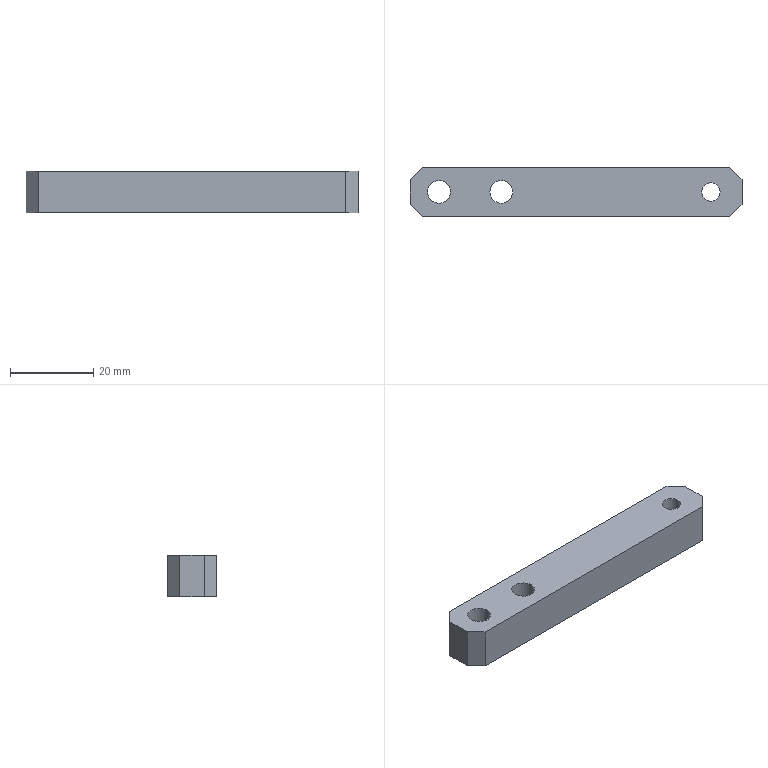Part | STEP file | 11-FG-B06711 | 1 solid | 27 faces | box 80 x 12 x 10 mm | volume 7960 mm3 | cylinder 14 | plane 13 | commonest cylinder face diameters 5.5 x4 10 x4 3.3 x2 4.4 x2 8 x2
STEP:
#1=CARTESIAN_POINT('',(12.,6.,5.4));
#2=VERTEX_POINT('',#1);
#3=CARTESIAN_POINT('',(2.,6.,5.4));
#4=VERTEX_POINT('',#3);
#5=CARTESIAN_POINT('',(7.,6.,5.4));
#6=DIRECTION('',(0.,0.,-1.));
#7=DIRECTION('',(-1.,0.,0.));
#8=AXIS2_PLACEMENT_3D('',#5,#6,#7);
#9=CIRCLE('',#8,5.);
#10=EDGE_CURVE('',#2,#4,#9,.T.);
#11=ORIENTED_EDGE('',*,*,#10,.F.);
#12=CARTESIAN_POINT('',(12.,6.,0.));
#13=VERTEX_POINT('',#12);
#14=CARTESIAN_POINT('',(12.,6.,0.));
#15=DIRECTION('',(0.,0.,-1.));
#16=VECTOR('',#15,1000.);
#17=LINE('',#14,#16);
#18=EDGE_CURVE('',#2,#13,#17,.T.);
#19=ORIENTED_EDGE('',*,*,#18,.T.);
#20=CARTESIAN_POINT('',(2.,6.,0.));
#21=VERTEX_POINT('',#20);
#22=CARTESIAN_POINT('',(7.,6.,0.));
#23=DIRECTION('',(0.,0.,-1.));
#24=DIRECTION('',(-1.,0.,0.));
#25=AXIS2_PLACEMENT_3D('',#22,#23,#24);
#26=CIRCLE('',#25,5.);
#27=EDGE_CURVE('',#13,#21,#26,.T.);
#28=ORIENTED_EDGE('',*,*,#27,.T.);
#29=CARTESIAN_POINT('',(2.,6.,0.));
#30=DIRECTION('',(0.,0.,-1.));
#31=VECTOR('',#30,1000.);
#32=LINE('',#29,#31);
#33=EDGE_CURVE('',#4,#21,#32,.T.);
#34=ORIENTED_EDGE('',*,*,#33,.F.);
#35=EDGE_LOOP('',(#11,#19,#28,#34));
#36=FACE_OUTER_BOUND('',#35,.T.);
#37=CARTESIAN_POINT('',(7.,6.,0.));
#38=DIRECTION('',(0.,0.,-1.));
#39=DIRECTION('',(-1.,0.,0.));
#40=AXIS2_PLACEMENT_3D('',#37,#38,#39);
#41=CYLINDRICAL_SURFACE('',#40,5.);
#42=ADVANCED_FACE('',(#36),#41,.F.);
#43=CARTESIAN_POINT('',(9.75,6.,10.));
#44=VERTEX_POINT('',#43);
#45=CARTESIAN_POINT('',(4.25,6.,10.));
#46=VERTEX_POINT('',#45);
#47=CARTESIAN_POINT('',(7.,6.,10.));
#48=DIRECTION('',(0.,0.,-1.));
#49=DIRECTION('',(-1.,0.,0.));
#50=AXIS2_PLACEMENT_3D('',#47,#48,#49);
#51=CIRCLE('',#50,2.75);
#52=EDGE_CURVE('',#44,#46,#51,.T.);
#53=ORIENTED_EDGE('',*,*,#52,.F.);
#54=CARTESIAN_POINT('',(9.75,6.,5.4));
#55=VERTEX_POINT('',#54);
#56=CARTESIAN_POINT('',(9.75,6.,0.));
#57=DIRECTION('',(0.,0.,-1.));
#58=VECTOR('',#57,1000.);
#59=LINE('',#56,#58);
#60=EDGE_CURVE('',#44,#55,#59,.T.);
#61=ORIENTED_EDGE('',*,*,#60,.T.);
#62=CARTESIAN_POINT('',(4.25,6.,5.4));
#63=VERTEX_POINT('',#62);
#64=CARTESIAN_POINT('',(7.,6.,5.4));
#65=DIRECTION('',(0.,0.,-1.));
#66=DIRECTION('',(-1.,0.,0.));
#67=AXIS2_PLACEMENT_3D('',#64,#65,#66);
#68=CIRCLE('',#67,2.75);
#69=EDGE_CURVE('',#55,#63,#68,.T.);
#70=ORIENTED_EDGE('',*,*,#69,.T.);
#71=CARTESIAN_POINT('',(4.25,6.,0.));
#72=DIRECTION('',(0.,0.,-1.));
#73=VECTOR('',#72,1000.);
#74=LINE('',#71,#73);
#75=EDGE_CURVE('',#46,#63,#74,.T.);
#76=ORIENTED_EDGE('',*,*,#75,.F.);
#77=EDGE_LOOP('',(#53,#61,#70,#76));
#78=FACE_OUTER_BOUND('',#77,.T.);
#79=CARTESIAN_POINT('',(7.,6.,0.));
#80=DIRECTION('',(0.,0.,-1.));
#81=DIRECTION('',(-1.,0.,0.));
#82=AXIS2_PLACEMENT_3D('',#79,#80,#81);
#83=CYLINDRICAL_SURFACE('',#82,2.75);
#84=ADVANCED_FACE('',(#78),#83,.F.);
#85=CARTESIAN_POINT('',(27.,6.,5.4));
#86=VERTEX_POINT('',#85);
#87=CARTESIAN_POINT('',(17.,6.,5.4));
#88=VERTEX_POINT('',#87);
#89=CARTESIAN_POINT('',(22.,6.,5.4));
#90=DIRECTION('',(0.,0.,-1.));
#91=DIRECTION('',(-1.,0.,0.));
#92=AXIS2_PLACEMENT_3D('',#89,#90,#91);
#93=CIRCLE('',#92,5.);
#94=EDGE_CURVE('',#86,#88,#93,.T.);
#95=ORIENTED_EDGE('',*,*,#94,.F.);
#96=CARTESIAN_POINT('',(27.,6.,0.));
#97=VERTEX_POINT('',#96);
#98=CARTESIAN_POINT('',(27.,6.,0.));
#99=DIRECTION('',(0.,0.,-1.));
#100=VECTOR('',#99,1000.);
#101=LINE('',#98,#100);
#102=EDGE_CURVE('',#86,#97,#101,.T.);
#103=ORIENTED_EDGE('',*,*,#102,.T.);
#104=CARTESIAN_POINT('',(17.,6.,0.));
#105=VERTEX_POINT('',#104);
#106=CARTESIAN_POINT('',(22.,6.,0.));
#107=DIRECTION('',(0.,0.,-1.));
#108=DIRECTION('',(-1.,0.,0.));
#109=AXIS2_PLACEMENT_3D('',#106,#107,#108);
#110=CIRCLE('',#109,5.);
#111=EDGE_CURVE('',#97,#105,#110,.T.);
#112=ORIENTED_EDGE('',*,*,#111,.T.);
#113=CARTESIAN_POINT('',(17.,6.,0.));
#114=DIRECTION('',(0.,0.,-1.));
#115=VECTOR('',#114,1000.);
#116=LINE('',#113,#115);
#117=EDGE_CURVE('',#88,#105,#116,.T.);
#118=ORIENTED_EDGE('',*,*,#117,.F.);
#119=EDGE_LOOP('',(#95,#103,#112,#118));
#120=FACE_OUTER_BOUND('',#119,.T.);
#121=CARTESIAN_POINT('',(22.,6.,0.));
#122=DIRECTION('',(0.,0.,-1.));
#123=DIRECTION('',(-1.,0.,0.));
#124=AXIS2_PLACEMENT_3D('',#121,#122,#123);
#125=CYLINDRICAL_SURFACE('',#124,5.);
#126=ADVANCED_FACE('',(#120),#125,.F.);
#127=CARTESIAN_POINT('',(24.75,6.,10.));
#128=VERTEX_POINT('',#127);
#129=CARTESIAN_POINT('',(19.25,6.,10.));
#130=VERTEX_POINT('',#129);
#131=CARTESIAN_POINT('',(22.,6.,10.));
#132=DIRECTION('',(0.,0.,-1.));
#133=DIRECTION('',(-1.,0.,0.));
#134=AXIS2_PLACEMENT_3D('',#131,#132,#133);
#135=CIRCLE('',#134,2.75);
#136=EDGE_CURVE('',#128,#130,#135,.T.);
#137=ORIENTED_EDGE('',*,*,#136,.F.);
#138=CARTESIAN_POINT('',(24.75,6.,5.4));
#139=VERTEX_POINT('',#138);
#140=CARTESIAN_POINT('',(24.75,6.,0.));
#141=DIRECTION('',(0.,0.,-1.));
#142=VECTOR('',#141,1000.);
#143=LINE('',#140,#142);
#144=EDGE_CURVE('',#128,#139,#143,.T.);
#145=ORIENTED_EDGE('',*,*,#144,.T.);
#146=CARTESIAN_POINT('',(19.25,6.,5.4));
#147=VERTEX_POINT('',#146);
#148=CARTESIAN_POINT('',(22.,6.,5.4));
#149=DIRECTION('',(0.,0.,-1.));
#150=DIRECTION('',(-1.,0.,0.));
#151=AXIS2_PLACEMENT_3D('',#148,#149,#150);
#152=CIRCLE('',#151,2.75);
#153=EDGE_CURVE('',#139,#147,#152,.T.);
#154=ORIENTED_EDGE('',*,*,#153,.T.);
#155=CARTESIAN_POINT('',(19.25,6.,0.));
#156=DIRECTION('',(0.,0.,-1.));
#157=VECTOR('',#156,1000.);
#158=LINE('',#155,#157);
#159=EDGE_CURVE('',#130,#147,#158,.T.);
#160=ORIENTED_EDGE('',*,*,#159,.F.);
#161=EDGE_LOOP('',(#137,#145,#154,#160));
#162=FACE_OUTER_BOUND('',#161,.T.);
#163=CARTESIAN_POINT('',(22.,6.,0.));
#164=DIRECTION('',(0.,0.,-1.));
#165=DIRECTION('',(-1.,0.,0.));
#166=AXIS2_PLACEMENT_3D('',#163,#164,#165);
#167=CYLINDRICAL_SURFACE('',#166,2.75);
#168=ADVANCED_FACE('',(#162),#167,.F.);
#169=CARTESIAN_POINT('',(76.5,6.,5.15));
#170=VERTEX_POINT('',#169);
#171=CARTESIAN_POINT('',(76.5,6.,1.85));
#172=VERTEX_POINT('',#171);
#173=CARTESIAN_POINT('',(76.5,6.,5.15));
#174=CARTESIAN_POINT('',(76.5,5.891,5.15));
#175=CARTESIAN_POINT('',(76.495,5.781,5.139));
#176=CARTESIAN_POINT('',(76.478,5.567,5.096));
#177=CARTESIAN_POINT('',(76.465,5.464,5.064));
#178=CARTESIAN_POINT('',(76.417,5.165,4.939));
#179=CARTESIAN_POINT('',(76.372,4.984,4.818));
#180=CARTESIAN_POINT('',(76.303,4.756,4.59));
#181=CARTESIAN_POINT('',(76.28,4.689,4.508));
#182=CARTESIAN_POINT('',(76.236,4.57,4.33));
#183=CARTESIAN_POINT('',(76.216,4.519,4.234));
#184=CARTESIAN_POINT('',(76.182,4.436,4.035));
#185=CARTESIAN_POINT('',(76.168,4.404,3.933));
#186=CARTESIAN_POINT('',(76.149,4.361,3.72));
#187=CARTESIAN_POINT('',(76.144,4.35,3.609));
#188=CARTESIAN_POINT('',(76.144,4.35,3.283));
#189=CARTESIAN_POINT('',(76.165,4.394,3.064));
#190=CARTESIAN_POINT('',(76.216,4.518,2.766));
#191=CARTESIAN_POINT('',(76.236,4.57,2.67));
#192=CARTESIAN_POINT('',(76.28,4.689,2.492));
#193=CARTESIAN_POINT('',(76.303,4.757,2.41));
#194=CARTESIAN_POINT('',(76.349,4.908,2.258));
#195=CARTESIAN_POINT('',(76.372,4.992,2.189));
#196=CARTESIAN_POINT('',(76.414,5.169,2.071));
#197=CARTESIAN_POINT('',(76.433,5.263,2.02));
#198=CARTESIAN_POINT('',(76.482,5.565,1.893));
#199=CARTESIAN_POINT('',(76.5,5.779,1.85));
#200=CARTESIAN_POINT('',(76.5,6.,1.85));
#201=B_SPLINE_CURVE_WITH_KNOTS('',3,(#173,#174,#175,#176,#177,#178,#179,#180,#181,#182,#183,#184,#185,#186,#187,#188,#189,#190,#191,#192,#193,#194,#195,#196,#197,#198,#199,#200),.UNSPECIFIED.,.F.,.F.,(4,2,2,2,2,2,2,2,2,2,2,2,2,4),(0.005218,0.005543,0.005869,0.006521,0.006847,0.007173,0.007499,0.007824,0.008476,0.008802,0.009128,0.009454,0.009779,0.01043),.UNSPECIFIED.);
#202=EDGE_CURVE('',#170,#172,#201,.T.);
#203=ORIENTED_EDGE('',*,*,#202,.F.);
#204=CARTESIAN_POINT('',(80.,6.,5.15));
#205=VERTEX_POINT('',#204);
#206=CARTESIAN_POINT('',(80.,6.,5.15));
#207=DIRECTION('',(1.,0.,0.));
#208=VECTOR('',#207,1000.);
#209=LINE('',#206,#208);
#210=EDGE_CURVE('',#170,#205,#209,.T.);
#211=ORIENTED_EDGE('',*,*,#210,.T.);
#212=CARTESIAN_POINT('',(80.,6.,1.85));
#213=VERTEX_POINT('',#212);
#214=CARTESIAN_POINT('',(80.,6.,3.5));
#215=DIRECTION('',(1.,0.,0.));
#216=DIRECTION('',(0.,0.,-1.));
#217=AXIS2_PLACEMENT_3D('',#214,#215,#216);
#218=CIRCLE('',#217,1.65);
#219=EDGE_CURVE('',#205,#213,#218,.T.);
#220=ORIENTED_EDGE('',*,*,#219,.T.);
#221=CARTESIAN_POINT('',(80.,6.,1.85));
#222=DIRECTION('',(1.,0.,0.));
#223=VECTOR('',#222,1000.);
#224=LINE('',#221,#223);
#225=EDGE_CURVE('',#172,#213,#224,.T.);
#226=ORIENTED_EDGE('',*,*,#225,.F.);
#227=EDGE_LOOP('',(#203,#211,#220,#226));
#228=FACE_OUTER_BOUND('',#227,.T.);
#229=CARTESIAN_POINT('',(80.,6.,3.5));
#230=DIRECTION('',(1.,0.,0.));
#231=DIRECTION('',(0.,0.,-1.));
#232=AXIS2_PLACEMENT_3D('',#229,#230,#231);
#233=CYLINDRICAL_SURFACE('',#232,1.65);
#234=ADVANCED_FACE('',(#228),#233,.F.);
#235=CARTESIAN_POINT('',(74.7,6.,6.));
#236=VERTEX_POINT('',#235);
#237=CARTESIAN_POINT('',(70.3,6.,6.));
#238=VERTEX_POINT('',#237);
#239=CARTESIAN_POINT('',(72.5,6.,6.));
#240=DIRECTION('',(0.,0.,-1.));
#241=DIRECTION('',(-1.,0.,0.));
#242=AXIS2_PLACEMENT_3D('',#239,#240,#241);
#243=CIRCLE('',#242,2.2);
#244=EDGE_CURVE('',#236,#238,#243,.T.);
#245=ORIENTED_EDGE('',*,*,#244,.T.);
#246=CARTESIAN_POINT('',(70.3,6.,10.));
#247=VERTEX_POINT('',#246);
#248=CARTESIAN_POINT('',(70.3,6.,10.));
#249=DIRECTION('',(0.,0.,1.));
#250=VECTOR('',#249,1000.);
#251=LINE('',#248,#250);
#252=EDGE_CURVE('',#238,#247,#251,.T.);
#253=ORIENTED_EDGE('',*,*,#252,.T.);
#254=CARTESIAN_POINT('',(74.7,6.,10.));
#255=VERTEX_POINT('',#254);
#256=CARTESIAN_POINT('',(72.5,6.,10.));
#257=DIRECTION('',(0.,0.,1.));
#258=DIRECTION('',(1.,0.,0.));
#259=AXIS2_PLACEMENT_3D('',#256,#257,#258);
#260=CIRCLE('',#259,2.2);
#261=EDGE_CURVE('',#247,#255,#260,.T.);
#262=ORIENTED_EDGE('',*,*,#261,.T.);
#263=CARTESIAN_POINT('',(74.7,6.,10.));
#264=DIRECTION('',(0.,0.,1.));
#265=VECTOR('',#264,1000.);
#266=LINE('',#263,#265);
#267=EDGE_CURVE('',#236,#255,#266,.T.);
#268=ORIENTED_EDGE('',*,*,#267,.F.);
#269=EDGE_LOOP('',(#245,#253,#262,#268));
#270=FACE_OUTER_BOUND('',#269,.T.);
#271=CARTESIAN_POINT('',(72.5,6.,10.));
#272=DIRECTION('',(0.,0.,1.));
#273=DIRECTION('',(1.,0.,0.));
#274=AXIS2_PLACEMENT_3D('',#271,#272,#273);
#275=CYLINDRICAL_SURFACE('',#274,2.2);
#276=ADVANCED_FACE('',(#270),#275,.F.);
#277=CARTESIAN_POINT('',(76.5,6.,6.));
#278=VERTEX_POINT('',#277);
#279=CARTESIAN_POINT('',(68.5,6.,6.));
#280=VERTEX_POINT('',#279);
#281=CARTESIAN_POINT('',(72.5,6.,6.));
#282=DIRECTION('',(0.,0.,-1.));
#283=DIRECTION('',(-1.,0.,0.));
#284=AXIS2_PLACEMENT_3D('',#281,#282,#283);
#285=CIRCLE('',#284,4.);
#286=EDGE_CURVE('',#278,#280,#285,.T.);
#287=ORIENTED_EDGE('',*,*,#286,.F.);
#288=CARTESIAN_POINT('',(76.5,6.,6.));
#289=DIRECTION('',(0.,0.,-1.));
#290=VECTOR('',#289,1000.);
#291=LINE('',#288,#290);
#292=EDGE_CURVE('',#278,#170,#291,.T.);
#293=ORIENTED_EDGE('',*,*,#292,.T.);
#294=ORIENTED_EDGE('',*,*,#202,.T.);
#295=CARTESIAN_POINT('',(76.5,6.,0.));
#296=VERTEX_POINT('',#295);
#297=CARTESIAN_POINT('',(76.5,6.,6.));
#298=DIRECTION('',(0.,0.,-1.));
#299=VECTOR('',#298,1000.);
#300=LINE('',#297,#299);
#301=EDGE_CURVE('',#172,#296,#300,.T.);
#302=ORIENTED_EDGE('',*,*,#301,.T.);
#303=CARTESIAN_POINT('',(68.5,6.,0.));
#304=VERTEX_POINT('',#303);
#305=CARTESIAN_POINT('',(72.5,6.,0.));
#306=DIRECTION('',(0.,0.,-1.));
#307=DIRECTION('',(-1.,0.,0.));
#308=AXIS2_PLACEMENT_3D('',#305,#306,#307);
#309=CIRCLE('',#308,4.);
#310=EDGE_CURVE('',#296,#304,#309,.T.);
#311=ORIENTED_EDGE('',*,*,#310,.T.);
#312=CARTESIAN_POINT('',(68.5,6.,6.));
#313=DIRECTION('',(0.,0.,-1.));
#314=VECTOR('',#313,1000.);
#315=LINE('',#312,#314);
#316=EDGE_CURVE('',#280,#304,#315,.T.);
#317=ORIENTED_EDGE('',*,*,#316,.F.);
#318=EDGE_LOOP('',(#287,#293,#294,#302,#311,#317));
#319=FACE_OUTER_BOUND('',#318,.T.);
#320=CARTESIAN_POINT('',(72.5,6.,6.));
#321=DIRECTION('',(0.,0.,-1.));
#322=DIRECTION('',(-1.,0.,0.));
#323=AXIS2_PLACEMENT_3D('',#320,#321,#322);
#324=CYLINDRICAL_SURFACE('',#323,4.);
#325=ADVANCED_FACE('',(#319),#324,.F.);
#326=CARTESIAN_POINT('',(0.,9.,0.));
#327=VERTEX_POINT('',#326);
#328=CARTESIAN_POINT('',(0.,3.,0.));
#329=VERTEX_POINT('',#328);
#330=CARTESIAN_POINT('',(0.,0.,0.));
#331=DIRECTION('',(0.,-1.,0.));
#332=VECTOR('',#331,1000.);
#333=LINE('',#330,#332);
#334=EDGE_CURVE('',#327,#329,#333,.T.);
#335=ORIENTED_EDGE('',*,*,#334,.T.);
#336=CARTESIAN_POINT('',(0.,3.,10.));
#337=VERTEX_POINT('',#336);
#338=CARTESIAN_POINT('',(0.,3.,10.));
#339=DIRECTION('',(0.,0.,1.));
#340=VECTOR('',#339,1000.);
#341=LINE('',#338,#340);
#342=EDGE_CURVE('',#329,#337,#341,.T.);
#343=ORIENTED_EDGE('',*,*,#342,.T.);
#344=CARTESIAN_POINT('',(0.,9.,10.));
#345=VERTEX_POINT('',#344);
#346=CARTESIAN_POINT('',(0.,0.,10.));
#347=DIRECTION('',(0.,-1.,0.));
#348=VECTOR('',#347,1000.);
#349=LINE('',#346,#348);
#350=EDGE_CURVE('',#345,#337,#349,.T.);
#351=ORIENTED_EDGE('',*,*,#350,.F.);
#352=CARTESIAN_POINT('',(0.,9.,10.));
#353=DIRECTION('',(0.,0.,-1.));
#354=VECTOR('',#353,1000.);
#355=LINE('',#352,#354);
#356=EDGE_CURVE('',#345,#327,#355,.T.);
#357=ORIENTED_EDGE('',*,*,#356,.T.);
#358=EDGE_LOOP('',(#335,#343,#351,#357));
#359=FACE_OUTER_BOUND('',#358,.T.);
#360=CARTESIAN_POINT('',(0.,0.,10.));
#361=DIRECTION('',(1.,0.,0.));
#362=DIRECTION('',(0.,0.,-1.));
#363=AXIS2_PLACEMENT_3D('',#360,#361,#362);
#364=PLANE('',#363);
#365=ADVANCED_FACE('',(#359),#364,.F.);
#366=CARTESIAN_POINT('',(3.,0.,0.));
#367=VERTEX_POINT('',#366);
#368=CARTESIAN_POINT('',(77.,0.,0.));
#369=VERTEX_POINT('',#368);
#370=CARTESIAN_POINT('',(0.,0.,0.));
#371=DIRECTION('',(1.,0.,0.));
#372=VECTOR('',#371,1000.);
#373=LINE('',#370,#372);
#374=EDGE_CURVE('',#367,#369,#373,.T.);
#375=ORIENTED_EDGE('',*,*,#374,.T.);
#376=CARTESIAN_POINT('',(77.,0.,10.));
#377=VERTEX_POINT('',#376);
#378=CARTESIAN_POINT('',(77.,0.,10.));
#379=DIRECTION('',(0.,0.,1.));
#380=VECTOR('',#379,1000.);
#381=LINE('',#378,#380);
#382=EDGE_CURVE('',#369,#377,#381,.T.);
#383=ORIENTED_EDGE('',*,*,#382,.T.);
#384=CARTESIAN_POINT('',(3.,0.,10.));
#385=VERTEX_POINT('',#384);
#386=CARTESIAN_POINT('',(0.,0.,10.));
#387=DIRECTION('',(1.,0.,0.));
#388=VECTOR('',#387,1000.);
#389=LINE('',#386,#388);
#390=EDGE_CURVE('',#385,#377,#389,.T.);
#391=ORIENTED_EDGE('',*,*,#390,.F.);
#392=CARTESIAN_POINT('',(3.,0.,10.));
#393=DIRECTION('',(0.,0.,-1.));
#394=VECTOR('',#393,1000.);
#395=LINE('',#392,#394);
#396=EDGE_CURVE('',#385,#367,#395,.T.);
#397=ORIENTED_EDGE('',*,*,#396,.T.);
#398=EDGE_LOOP('',(#375,#383,#391,#397));
#399=FACE_OUTER_BOUND('',#398,.T.);
#400=CARTESIAN_POINT('',(0.,0.,10.));
#401=DIRECTION('',(0.,1.,0.));
#402=DIRECTION('',(0.,0.,1.));
#403=AXIS2_PLACEMENT_3D('',#400,#401,#402);
#404=PLANE('',#403);
#405=ADVANCED_FACE('',(#399),#404,.F.);
#406=CARTESIAN_POINT('',(80.,6.,3.5));
#407=DIRECTION('',(1.,0.,0.));
#408=DIRECTION('',(0.,0.,-1.));
#409=AXIS2_PLACEMENT_3D('',#406,#407,#408);
#410=CIRCLE('',#409,1.65);
#411=EDGE_CURVE('',#213,#205,#410,.T.);
#412=ORIENTED_EDGE('',*,*,#411,.F.);
#413=ORIENTED_EDGE('',*,*,#219,.F.);
#414=EDGE_LOOP('',(#412,#413));
#415=FACE_BOUND('',#414,.T.);
#416=CARTESIAN_POINT('',(80.,3.,10.));
#417=VERTEX_POINT('',#416);
#418=CARTESIAN_POINT('',(80.,9.,10.));
#419=VERTEX_POINT('',#418);
#420=CARTESIAN_POINT('',(80.,0.,10.));
#421=DIRECTION('',(0.,1.,0.));
#422=VECTOR('',#421,1000.);
#423=LINE('',#420,#422);
#424=EDGE_CURVE('',#417,#419,#423,.T.);
#425=ORIENTED_EDGE('',*,*,#424,.F.);
#426=CARTESIAN_POINT('',(80.,3.,0.));
#427=VERTEX_POINT('',#426);
#428=CARTESIAN_POINT('',(80.,3.,10.));
#429=DIRECTION('',(0.,0.,-1.));
#430=VECTOR('',#429,1000.);
#431=LINE('',#428,#430);
#432=EDGE_CURVE('',#417,#427,#431,.T.);
#433=ORIENTED_EDGE('',*,*,#432,.T.);
#434=CARTESIAN_POINT('',(80.,9.,0.));
#435=VERTEX_POINT('',#434);
#436=CARTESIAN_POINT('',(80.,0.,0.));
#437=DIRECTION('',(0.,1.,0.));
#438=VECTOR('',#437,1000.);
#439=LINE('',#436,#438);
#440=EDGE_CURVE('',#427,#435,#439,.T.);
#441=ORIENTED_EDGE('',*,*,#440,.T.);
#442=CARTESIAN_POINT('',(80.,9.,10.));
#443=DIRECTION('',(0.,0.,1.));
#444=VECTOR('',#443,1000.);
#445=LINE('',#442,#444);
#446=EDGE_CURVE('',#435,#419,#445,.T.);
#447=ORIENTED_EDGE('',*,*,#446,.T.);
#448=EDGE_LOOP('',(#425,#433,#441,#447));
#449=FACE_OUTER_BOUND('',#448,.T.);
#450=CARTESIAN_POINT('',(80.,0.,10.));
#451=DIRECTION('',(-1.,0.,0.));
#452=DIRECTION('',(0.,0.,1.));
#453=AXIS2_PLACEMENT_3D('',#450,#451,#452);
#454=PLANE('',#453);
#455=ADVANCED_FACE('',(#415,#449),#454,.F.);
#456=CARTESIAN_POINT('',(77.,12.,10.));
#457=VERTEX_POINT('',#456);
#458=CARTESIAN_POINT('',(3.,12.,10.));
#459=VERTEX_POINT('',#458);
#460=CARTESIAN_POINT('',(0.,12.,10.));
#461=DIRECTION('',(-1.,0.,0.));
#462=VECTOR('',#461,1000.);
#463=LINE('',#460,#462);
#464=EDGE_CURVE('',#457,#459,#463,.T.);
#465=ORIENTED_EDGE('',*,*,#464,.F.);
#466=CARTESIAN_POINT('',(77.,12.,0.));
#467=VERTEX_POINT('',#466);
#468=CARTESIAN_POINT('',(77.,12.,10.));
#469=DIRECTION('',(0.,0.,-1.));
#470=VECTOR('',#469,1000.);
#471=LINE('',#468,#470);
#472=EDGE_CURVE('',#457,#467,#471,.T.);
#473=ORIENTED_EDGE('',*,*,#472,.T.);
#474=CARTESIAN_POINT('',(3.,12.,0.));
#475=VERTEX_POINT('',#474);
#476=CARTESIAN_POINT('',(0.,12.,0.));
#477=DIRECTION('',(-1.,0.,0.));
#478=VECTOR('',#477,1000.);
#479=LINE('',#476,#478);
#480=EDGE_CURVE('',#467,#475,#479,.T.);
#481=ORIENTED_EDGE('',*,*,#480,.T.);
#482=CARTESIAN_POINT('',(3.,12.,10.));
#483=DIRECTION('',(0.,0.,1.));
#484=VECTOR('',#483,1000.);
#485=LINE('',#482,#484);
#486=EDGE_CURVE('',#475,#459,#485,.T.);
#487=ORIENTED_EDGE('',*,*,#486,.T.);
#488=EDGE_LOOP('',(#465,#473,#481,#487));
#489=FACE_OUTER_BOUND('',#488,.T.);
#490=CARTESIAN_POINT('',(0.,12.,10.));
#491=DIRECTION('',(0.,-1.,0.));
#492=DIRECTION('',(0.,0.,-1.));
#493=AXIS2_PLACEMENT_3D('',#490,#491,#492);
#494=PLANE('',#493);
#495=ADVANCED_FACE('',(#489),#494,.F.);
#496=CARTESIAN_POINT('',(7.,6.,10.));
#497=DIRECTION('',(0.,0.,-1.));
#498=DIRECTION('',(-1.,0.,0.));
#499=AXIS2_PLACEMENT_3D('',#496,#497,#498);
#500=CIRCLE('',#499,2.75);
#501=EDGE_CURVE('',#46,#44,#500,.T.);
#502=ORIENTED_EDGE('',*,*,#501,.T.);
#503=ORIENTED_EDGE('',*,*,#52,.T.);
#504=EDGE_LOOP('',(#502,#503));
#505=FACE_BOUND('',#504,.T.);
#506=CARTESIAN_POINT('',(22.,6.,10.));
#507=DIRECTION('',(0.,0.,-1.));
#508=DIRECTION('',(-1.,0.,0.));
#509=AXIS2_PLACEMENT_3D('',#506,#507,#508);
#510=CIRCLE('',#509,2.75);
#511=EDGE_CURVE('',#130,#128,#510,.T.);
#512=ORIENTED_EDGE('',*,*,#511,.T.);
#513=ORIENTED_EDGE('',*,*,#136,.T.);
#514=EDGE_LOOP('',(#512,#513));
#515=FACE_BOUND('',#514,.T.);
#516=CARTESIAN_POINT('',(72.5,6.,10.));
#517=DIRECTION('',(0.,0.,1.));
#518=DIRECTION('',(1.,0.,0.));
#519=AXIS2_PLACEMENT_3D('',#516,#517,#518);
#520=CIRCLE('',#519,2.2);
#521=EDGE_CURVE('',#255,#247,#520,.T.);
#522=ORIENTED_EDGE('',*,*,#521,.F.);
#523=ORIENTED_EDGE('',*,*,#261,.F.);
#524=EDGE_LOOP('',(#522,#523));
#525=FACE_BOUND('',#524,.T.);
#526=ORIENTED_EDGE('',*,*,#390,.T.);
#527=CARTESIAN_POINT('',(80.,3.,10.));
#528=DIRECTION('',(0.7071,0.7071,0.));
#529=VECTOR('',#528,1000.);
#530=LINE('',#527,#529);
#531=EDGE_CURVE('',#377,#417,#530,.T.);
#532=ORIENTED_EDGE('',*,*,#531,.T.);
#533=ORIENTED_EDGE('',*,*,#424,.T.);
#534=CARTESIAN_POINT('',(77.,12.,10.));
#535=DIRECTION('',(-0.7071,0.7071,0.));
#536=VECTOR('',#535,1000.);
#537=LINE('',#534,#536);
#538=EDGE_CURVE('',#419,#457,#537,.T.);
#539=ORIENTED_EDGE('',*,*,#538,.T.);
#540=ORIENTED_EDGE('',*,*,#464,.T.);
#541=CARTESIAN_POINT('',(0.,9.,10.));
#542=DIRECTION('',(-0.7071,-0.7071,0.));
#543=VECTOR('',#542,1000.);
#544=LINE('',#541,#543);
#545=EDGE_CURVE('',#459,#345,#544,.T.);
#546=ORIENTED_EDGE('',*,*,#545,.T.);
#547=ORIENTED_EDGE('',*,*,#350,.T.);
#548=CARTESIAN_POINT('',(3.,0.,10.));
#549=DIRECTION('',(0.7071,-0.7071,0.));
#550=VECTOR('',#549,1000.);
#551=LINE('',#548,#550);
#552=EDGE_CURVE('',#337,#385,#551,.T.);
#553=ORIENTED_EDGE('',*,*,#552,.T.);
#554=EDGE_LOOP('',(#526,#532,#533,#539,#540,#546,#547,#553));
#555=FACE_OUTER_BOUND('',#554,.T.);
#556=CARTESIAN_POINT('',(0.,12.,10.));
#557=DIRECTION('',(0.,0.,-1.));
#558=DIRECTION('',(-1.,0.,0.));
#559=AXIS2_PLACEMENT_3D('',#556,#557,#558);
#560=PLANE('',#559);
#561=ADVANCED_FACE('',(#505,#515,#525,#555),#560,.F.);
#562=CARTESIAN_POINT('',(7.,6.,0.));
#563=DIRECTION('',(0.,0.,-1.));
#564=DIRECTION('',(-1.,0.,0.));
#565=AXIS2_PLACEMENT_3D('',#562,#563,#564);
#566=CIRCLE('',#565,5.);
#567=EDGE_CURVE('',#21,#13,#566,.T.);
#568=ORIENTED_EDGE('',*,*,#567,.F.);
#569=ORIENTED_EDGE('',*,*,#27,.F.);
#570=EDGE_LOOP('',(#568,#569));
#571=FACE_BOUND('',#570,.T.);
#572=CARTESIAN_POINT('',(22.,6.,0.));
#573=DIRECTION('',(0.,0.,-1.));
#574=DIRECTION('',(-1.,0.,0.));
#575=AXIS2_PLACEMENT_3D('',#572,#573,#574);
#576=CIRCLE('',#575,5.);
#577=EDGE_CURVE('',#105,#97,#576,.T.);
#578=ORIENTED_EDGE('',*,*,#577,.F.);
#579=ORIENTED_EDGE('',*,*,#111,.F.);
#580=EDGE_LOOP('',(#578,#579));
#581=FACE_BOUND('',#580,.T.);
#582=CARTESIAN_POINT('',(72.5,6.,0.));
#583=DIRECTION('',(0.,0.,-1.));
#584=DIRECTION('',(-1.,0.,0.));
#585=AXIS2_PLACEMENT_3D('',#582,#583,#584);
#586=CIRCLE('',#585,4.);
#587=EDGE_CURVE('',#304,#296,#586,.T.);
#588=ORIENTED_EDGE('',*,*,#587,.F.);
#589=ORIENTED_EDGE('',*,*,#310,.F.);
#590=EDGE_LOOP('',(#588,#589));
#591=FACE_BOUND('',#590,.T.);
#592=ORIENTED_EDGE('',*,*,#440,.F.);
#593=CARTESIAN_POINT('',(44.5,-32.5,0.));
#594=DIRECTION('',(-0.7071,-0.7071,0.));
#595=VECTOR('',#594,1000.);
#596=LINE('',#593,#595);
#597=EDGE_CURVE('',#427,#369,#596,.T.);
#598=ORIENTED_EDGE('',*,*,#597,.T.);
#599=ORIENTED_EDGE('',*,*,#374,.F.);
#600=CARTESIAN_POINT('',(-4.5,7.5,0.));
#601=DIRECTION('',(-0.7071,0.7071,0.));
#602=VECTOR('',#601,1000.);
#603=LINE('',#600,#602);
#604=EDGE_CURVE('',#367,#329,#603,.T.);
#605=ORIENTED_EDGE('',*,*,#604,.T.);
#606=ORIENTED_EDGE('',*,*,#334,.F.);
#607=CARTESIAN_POINT('',(1.5,10.5,0.));
#608=DIRECTION('',(0.7071,0.7071,0.));
#609=VECTOR('',#608,1000.);
#610=LINE('',#607,#609);
#611=EDGE_CURVE('',#327,#475,#610,.T.);
#612=ORIENTED_EDGE('',*,*,#611,.T.);
#613=ORIENTED_EDGE('',*,*,#480,.F.);
#614=CARTESIAN_POINT('',(38.5,50.5,0.));
#615=DIRECTION('',(0.7071,-0.7071,0.));
#616=VECTOR('',#615,1000.);
#617=LINE('',#614,#616);
#618=EDGE_CURVE('',#467,#435,#617,.T.);
#619=ORIENTED_EDGE('',*,*,#618,.T.);
#620=EDGE_LOOP('',(#592,#598,#599,#605,#606,#612,#613,#619));
#621=FACE_OUTER_BOUND('',#620,.T.);
#622=CARTESIAN_POINT('',(0.,12.,0.));
#623=DIRECTION('',(0.,0.,-1.));
#624=DIRECTION('',(-1.,0.,0.));
#625=AXIS2_PLACEMENT_3D('',#622,#623,#624);
#626=PLANE('',#625);
#627=ADVANCED_FACE('',(#571,#581,#591,#621),#626,.T.);
#628=ORIENTED_EDGE('',*,*,#531,.F.);
#629=ORIENTED_EDGE('',*,*,#382,.F.);
#630=ORIENTED_EDGE('',*,*,#597,.F.);
#631=ORIENTED_EDGE('',*,*,#432,.F.);
#632=EDGE_LOOP('',(#628,#629,#630,#631));
#633=FACE_OUTER_BOUND('',#632,.T.);
#634=CARTESIAN_POINT('',(80.,3.,10.));
#635=DIRECTION('',(-0.7071,0.7071,0.));
#636=DIRECTION('',(-0.7071,-0.7071,0.));
#637=AXIS2_PLACEMENT_3D('',#634,#635,#636);
#638=PLANE('',#637);
#639=ADVANCED_FACE('',(#633),#638,.F.);
#640=ORIENTED_EDGE('',*,*,#538,.F.);
#641=ORIENTED_EDGE('',*,*,#446,.F.);
#642=ORIENTED_EDGE('',*,*,#618,.F.);
#643=ORIENTED_EDGE('',*,*,#472,.F.);
#644=EDGE_LOOP('',(#640,#641,#642,#643));
#645=FACE_OUTER_BOUND('',#644,.T.);
#646=CARTESIAN_POINT('',(77.,12.,10.));
#647=DIRECTION('',(-0.7071,-0.7071,0.));
#648=DIRECTION('',(0.7071,-0.7071,0.));
#649=AXIS2_PLACEMENT_3D('',#646,#647,#648);
#650=PLANE('',#649);
#651=ADVANCED_FACE('',(#645),#650,.F.);
#652=ORIENTED_EDGE('',*,*,#552,.F.);
#653=ORIENTED_EDGE('',*,*,#342,.F.);
#654=ORIENTED_EDGE('',*,*,#604,.F.);
#655=ORIENTED_EDGE('',*,*,#396,.F.);
#656=EDGE_LOOP('',(#652,#653,#654,#655));
#657=FACE_OUTER_BOUND('',#656,.T.);
#658=CARTESIAN_POINT('',(3.,0.,10.));
#659=DIRECTION('',(0.7071,0.7071,0.));
#660=DIRECTION('',(-0.7071,0.7071,0.));
#661=AXIS2_PLACEMENT_3D('',#658,#659,#660);
#662=PLANE('',#661);
#663=ADVANCED_FACE('',(#657),#662,.F.);
#664=ORIENTED_EDGE('',*,*,#545,.F.);
#665=ORIENTED_EDGE('',*,*,#486,.F.);
#666=ORIENTED_EDGE('',*,*,#611,.F.);
#667=ORIENTED_EDGE('',*,*,#356,.F.);
#668=EDGE_LOOP('',(#664,#665,#666,#667));
#669=FACE_OUTER_BOUND('',#668,.T.);
#670=CARTESIAN_POINT('',(0.,9.,10.));
#671=DIRECTION('',(0.7071,-0.7071,0.));
#672=DIRECTION('',(0.7071,0.7071,0.));
#673=AXIS2_PLACEMENT_3D('',#670,#671,#672);
#674=PLANE('',#673);
#675=ADVANCED_FACE('',(#669),#674,.F.);
#676=ORIENTED_EDGE('',*,*,#292,.F.);
#677=CARTESIAN_POINT('',(72.5,6.,6.));
#678=DIRECTION('',(0.,0.,-1.));
#679=DIRECTION('',(-1.,0.,0.));
#680=AXIS2_PLACEMENT_3D('',#677,#678,#679);
#681=CIRCLE('',#680,4.);
#682=EDGE_CURVE('',#280,#278,#681,.T.);
#683=ORIENTED_EDGE('',*,*,#682,.F.);
#684=ORIENTED_EDGE('',*,*,#316,.T.);
#685=ORIENTED_EDGE('',*,*,#587,.T.);
#686=ORIENTED_EDGE('',*,*,#301,.F.);
#687=CARTESIAN_POINT('',(76.5,6.,1.85));
#688=CARTESIAN_POINT('',(76.5,6.11,1.85));
#689=CARTESIAN_POINT('',(76.495,6.219,1.861));
#690=CARTESIAN_POINT('',(76.478,6.431,1.904));
#691=CARTESIAN_POINT('',(76.465,6.537,1.936));
#692=CARTESIAN_POINT('',(76.417,6.836,2.061));
#693=CARTESIAN_POINT('',(76.372,7.017,2.184));
#694=CARTESIAN_POINT('',(76.28,7.318,2.485));
#695=CARTESIAN_POINT('',(76.233,7.44,2.666));
#696=CARTESIAN_POINT('',(76.182,7.564,2.963));
#697=CARTESIAN_POINT('',(76.168,7.596,3.068));
#698=CARTESIAN_POINT('',(76.149,7.639,3.282));
#699=CARTESIAN_POINT('',(76.144,7.65,3.39));
#700=CARTESIAN_POINT('',(76.144,7.65,3.608));
#701=CARTESIAN_POINT('',(76.149,7.639,3.719));
#702=CARTESIAN_POINT('',(76.168,7.596,3.931));
#703=CARTESIAN_POINT('',(76.182,7.565,4.035));
#704=CARTESIAN_POINT('',(76.216,7.481,4.236));
#705=CARTESIAN_POINT('',(76.236,7.43,4.33));
#706=CARTESIAN_POINT('',(76.28,7.311,4.508));
#707=CARTESIAN_POINT('',(76.303,7.242,4.592));
#708=CARTESIAN_POINT('',(76.349,7.091,4.743));
#709=CARTESIAN_POINT('',(76.372,7.009,4.81));
#710=CARTESIAN_POINT('',(76.414,6.83,4.93));
#711=CARTESIAN_POINT('',(76.433,6.734,4.981));
#712=CARTESIAN_POINT('',(76.481,6.437,5.106));
#713=CARTESIAN_POINT('',(76.5,6.217,5.15));
#714=CARTESIAN_POINT('',(76.5,6.,5.15));
#715=B_SPLINE_CURVE_WITH_KNOTS('',3,(#687,#688,#689,#690,#691,#692,#693,#694,#695,#696,#697,#698,#699,#700,#701,#702,#703,#704,#705,#706,#707,#708,#709,#710,#711,#712,#713,#714),.UNSPECIFIED.,.F.,.F.,(4,2,2,2,2,2,2,2,2,2,2,2,2,4),(0.,0.0003261,0.0006522,0.001304,0.001957,0.002283,0.002609,0.002935,0.003261,0.003587,0.003913,0.004239,0.004565,0.005218),.UNSPECIFIED.);
#716=EDGE_CURVE('',#172,#170,#715,.T.);
#717=ORIENTED_EDGE('',*,*,#716,.T.);
#718=EDGE_LOOP('',(#676,#683,#684,#685,#686,#717));
#719=FACE_OUTER_BOUND('',#718,.T.);
#720=CARTESIAN_POINT('',(72.5,6.,6.));
#721=DIRECTION('',(0.,0.,-1.));
#722=DIRECTION('',(-1.,0.,0.));
#723=AXIS2_PLACEMENT_3D('',#720,#721,#722);
#724=CYLINDRICAL_SURFACE('',#723,4.);
#725=ADVANCED_FACE('',(#719),#724,.F.);
#726=ORIENTED_EDGE('',*,*,#244,.F.);
#727=CARTESIAN_POINT('',(72.5,6.,6.));
#728=DIRECTION('',(0.,0.,-1.));
#729=DIRECTION('',(-1.,0.,0.));
#730=AXIS2_PLACEMENT_3D('',#727,#728,#729);
#731=CIRCLE('',#730,2.2);
#732=EDGE_CURVE('',#238,#236,#731,.T.);
#733=ORIENTED_EDGE('',*,*,#732,.F.);
#734=EDGE_LOOP('',(#726,#733));
#735=FACE_BOUND('',#734,.T.);
#736=ORIENTED_EDGE('',*,*,#682,.T.);
#737=ORIENTED_EDGE('',*,*,#286,.T.);
#738=EDGE_LOOP('',(#736,#737));
#739=FACE_OUTER_BOUND('',#738,.T.);
#740=CARTESIAN_POINT('',(72.5,6.,6.));
#741=DIRECTION('',(0.,0.,-1.));
#742=DIRECTION('',(-1.,0.,0.));
#743=AXIS2_PLACEMENT_3D('',#740,#741,#742);
#744=PLANE('',#743);
#745=ADVANCED_FACE('',(#735,#739),#744,.T.);
#746=ORIENTED_EDGE('',*,*,#252,.F.);
#747=ORIENTED_EDGE('',*,*,#732,.T.);
#748=ORIENTED_EDGE('',*,*,#267,.T.);
#749=ORIENTED_EDGE('',*,*,#521,.T.);
#750=EDGE_LOOP('',(#746,#747,#748,#749));
#751=FACE_OUTER_BOUND('',#750,.T.);
#752=CARTESIAN_POINT('',(72.5,6.,10.));
#753=DIRECTION('',(0.,0.,1.));
#754=DIRECTION('',(1.,0.,0.));
#755=AXIS2_PLACEMENT_3D('',#752,#753,#754);
#756=CYLINDRICAL_SURFACE('',#755,2.2);
#757=ADVANCED_FACE('',(#751),#756,.F.);
#758=ORIENTED_EDGE('',*,*,#210,.F.);
#759=ORIENTED_EDGE('',*,*,#716,.F.);
#760=ORIENTED_EDGE('',*,*,#225,.T.);
#761=ORIENTED_EDGE('',*,*,#411,.T.);
#762=EDGE_LOOP('',(#758,#759,#760,#761));
#763=FACE_OUTER_BOUND('',#762,.T.);
#764=CARTESIAN_POINT('',(80.,6.,3.5));
#765=DIRECTION('',(1.,0.,0.));
#766=DIRECTION('',(0.,0.,-1.));
#767=AXIS2_PLACEMENT_3D('',#764,#765,#766);
#768=CYLINDRICAL_SURFACE('',#767,1.65);
#769=ADVANCED_FACE('',(#763),#768,.F.);
#770=ORIENTED_EDGE('',*,*,#144,.F.);
#771=ORIENTED_EDGE('',*,*,#511,.F.);
#772=ORIENTED_EDGE('',*,*,#159,.T.);
#773=CARTESIAN_POINT('',(22.,6.,5.4));
#774=DIRECTION('',(0.,0.,-1.));
#775=DIRECTION('',(-1.,0.,0.));
#776=AXIS2_PLACEMENT_3D('',#773,#774,#775);
#777=CIRCLE('',#776,2.75);
#778=EDGE_CURVE('',#147,#139,#777,.T.);
#779=ORIENTED_EDGE('',*,*,#778,.T.);
#780=EDGE_LOOP('',(#770,#771,#772,#779));
#781=FACE_OUTER_BOUND('',#780,.T.);
#782=CARTESIAN_POINT('',(22.,6.,0.));
#783=DIRECTION('',(0.,0.,-1.));
#784=DIRECTION('',(-1.,0.,0.));
#785=AXIS2_PLACEMENT_3D('',#782,#783,#784);
#786=CYLINDRICAL_SURFACE('',#785,2.75);
#787=ADVANCED_FACE('',(#781),#786,.F.);
#788=ORIENTED_EDGE('',*,*,#778,.F.);
#789=ORIENTED_EDGE('',*,*,#153,.F.);
#790=EDGE_LOOP('',(#788,#789));
#791=FACE_BOUND('',#790,.T.);
#792=CARTESIAN_POINT('',(22.,6.,5.4));
#793=DIRECTION('',(0.,0.,-1.));
#794=DIRECTION('',(-1.,0.,0.));
#795=AXIS2_PLACEMENT_3D('',#792,#793,#794);
#796=CIRCLE('',#795,5.);
#797=EDGE_CURVE('',#88,#86,#796,.T.);
#798=ORIENTED_EDGE('',*,*,#797,.T.);
#799=ORIENTED_EDGE('',*,*,#94,.T.);
#800=EDGE_LOOP('',(#798,#799));
#801=FACE_OUTER_BOUND('',#800,.T.);
#802=CARTESIAN_POINT('',(24.75,6.,5.4));
#803=DIRECTION('',(0.,0.,1.));
#804=DIRECTION('',(1.,0.,0.));
#805=AXIS2_PLACEMENT_3D('',#802,#803,#804);
#806=PLANE('',#805);
#807=ADVANCED_FACE('',(#791,#801),#806,.F.);
#808=ORIENTED_EDGE('',*,*,#102,.F.);
#809=ORIENTED_EDGE('',*,*,#797,.F.);
#810=ORIENTED_EDGE('',*,*,#117,.T.);
#811=ORIENTED_EDGE('',*,*,#577,.T.);
#812=EDGE_LOOP('',(#808,#809,#810,#811));
#813=FACE_OUTER_BOUND('',#812,.T.);
#814=CARTESIAN_POINT('',(22.,6.,0.));
#815=DIRECTION('',(0.,0.,-1.));
#816=DIRECTION('',(-1.,0.,0.));
#817=AXIS2_PLACEMENT_3D('',#814,#815,#816);
#818=CYLINDRICAL_SURFACE('',#817,5.);
#819=ADVANCED_FACE('',(#813),#818,.F.);
#820=ORIENTED_EDGE('',*,*,#60,.F.);
#821=ORIENTED_EDGE('',*,*,#501,.F.);
#822=ORIENTED_EDGE('',*,*,#75,.T.);
#823=CARTESIAN_POINT('',(7.,6.,5.4));
#824=DIRECTION('',(0.,0.,-1.));
#825=DIRECTION('',(-1.,0.,0.));
#826=AXIS2_PLACEMENT_3D('',#823,#824,#825);
#827=CIRCLE('',#826,2.75);
#828=EDGE_CURVE('',#63,#55,#827,.T.);
#829=ORIENTED_EDGE('',*,*,#828,.T.);
#830=EDGE_LOOP('',(#820,#821,#822,#829));
#831=FACE_OUTER_BOUND('',#830,.T.);
#832=CARTESIAN_POINT('',(7.,6.,0.));
#833=DIRECTION('',(0.,0.,-1.));
#834=DIRECTION('',(-1.,0.,0.));
#835=AXIS2_PLACEMENT_3D('',#832,#833,#834);
#836=CYLINDRICAL_SURFACE('',#835,2.75);
#837=ADVANCED_FACE('',(#831),#836,.F.);
#838=ORIENTED_EDGE('',*,*,#828,.F.);
#839=ORIENTED_EDGE('',*,*,#69,.F.);
#840=EDGE_LOOP('',(#838,#839));
#841=FACE_BOUND('',#840,.T.);
#842=CARTESIAN_POINT('',(7.,6.,5.4));
#843=DIRECTION('',(0.,0.,-1.));
#844=DIRECTION('',(-1.,0.,0.));
#845=AXIS2_PLACEMENT_3D('',#842,#843,#844);
#846=CIRCLE('',#845,5.);
#847=EDGE_CURVE('',#4,#2,#846,.T.);
#848=ORIENTED_EDGE('',*,*,#847,.T.);
#849=ORIENTED_EDGE('',*,*,#10,.T.);
#850=EDGE_LOOP('',(#848,#849));
#851=FACE_OUTER_BOUND('',#850,.T.);
#852=CARTESIAN_POINT('',(9.75,6.,5.4));
#853=DIRECTION('',(0.,0.,1.));
#854=DIRECTION('',(1.,0.,0.));
#855=AXIS2_PLACEMENT_3D('',#852,#853,#854);
#856=PLANE('',#855);
#857=ADVANCED_FACE('',(#841,#851),#856,.F.);
#858=ORIENTED_EDGE('',*,*,#18,.F.);
#859=ORIENTED_EDGE('',*,*,#847,.F.);
#860=ORIENTED_EDGE('',*,*,#33,.T.);
#861=ORIENTED_EDGE('',*,*,#567,.T.);
#862=EDGE_LOOP('',(#858,#859,#860,#861));
#863=FACE_OUTER_BOUND('',#862,.T.);
#864=CARTESIAN_POINT('',(7.,6.,0.));
#865=DIRECTION('',(0.,0.,-1.));
#866=DIRECTION('',(-1.,0.,0.));
#867=AXIS2_PLACEMENT_3D('',#864,#865,#866);
#868=CYLINDRICAL_SURFACE('',#867,5.);
#869=ADVANCED_FACE('',(#863),#868,.F.);
#870=CLOSED_SHELL('',(#42,#84,#126,#168,#234,#276,#325,#365,#405,#455,#495,#561,#627,#639,#651,#663,#675,#725,#745,#757,#769,#787,#807,#819,#837,#857,#869));
#871=MANIFOLD_SOLID_BREP('',#870);
#872=CARTESIAN_POINT('',(0.,0.,0.));
#873=DIRECTION('',(0.,0.,1.));
#874=DIRECTION('',(1.,0.,0.));
#875=AXIS2_PLACEMENT_3D('',#872,#873,#874);
#876=(LENGTH_UNIT()NAMED_UNIT(*)SI_UNIT(.MILLI.,.METRE.));
#877=UNCERTAINTY_MEASURE_WITH_UNIT(LENGTH_MEASURE(0.00001),#876,'','');
#878=(NAMED_UNIT(*)PLANE_ANGLE_UNIT()SI_UNIT($,.RADIAN.));
#879=(NAMED_UNIT(*)SI_UNIT($,.STERADIAN.)SOLID_ANGLE_UNIT());
#880=(GEOMETRIC_REPRESENTATION_CONTEXT(3)GLOBAL_UNCERTAINTY_ASSIGNED_CONTEXT((#877))GLOBAL_UNIT_ASSIGNED_CONTEXT((#876,#878,#879))REPRESENTATION_CONTEXT('',''));
#881=ADVANCED_BREP_SHAPE_REPRESENTATION('',(#871,#875),#880);